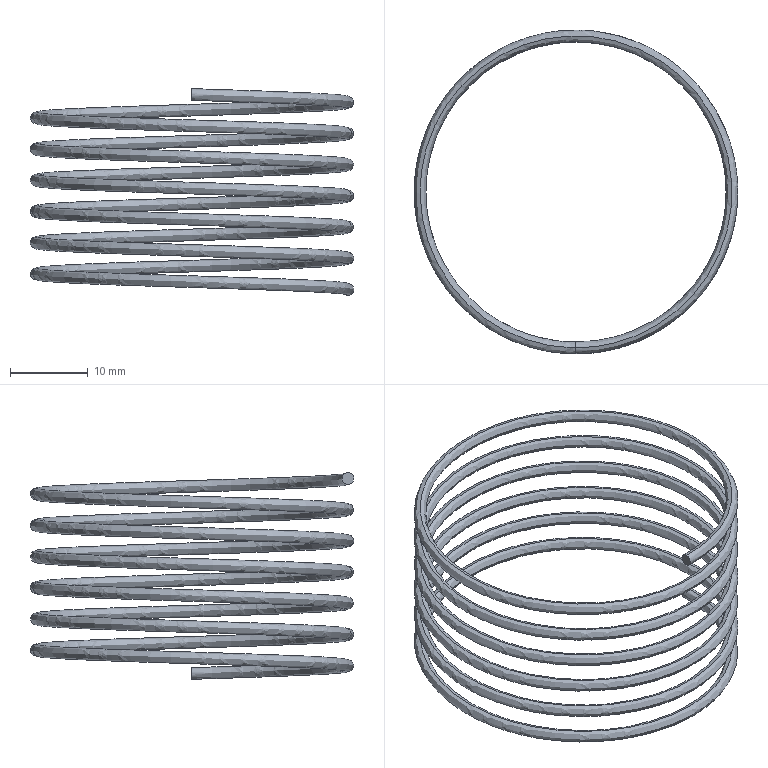Part | STEP file | Spring-circlip check | 1 solid | 4 faces | box 41.5 x 41.5 x 26.5 mm | volume 1389 mm3 | spline 2 | plane 2